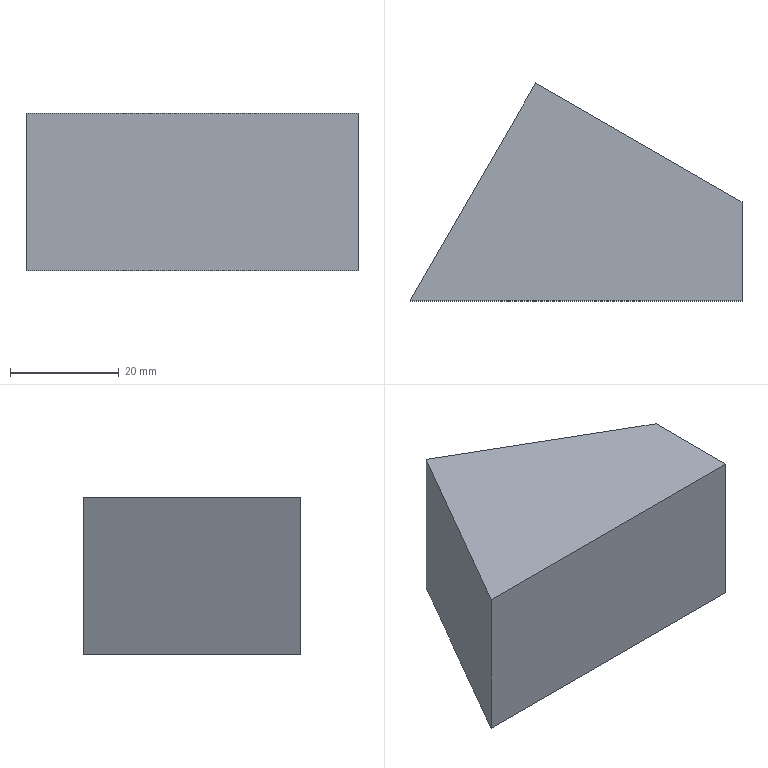Part | Creo | 1 solid | 6 faces | box 61.174 x 40.149 x 29 mm | volume 45647 mm3 | plane 6
STEP:
#1=CARTESIAN_POINT('',(9.022,228.213,-50.5));
#2=VERTEX_POINT('',#1);
#3=CARTESIAN_POINT('',(-28.972,250.149,-50.5));
#4=VERTEX_POINT('',#3);
#5=CARTESIAN_POINT('',(9.022,228.213,-50.5));
#6=DIRECTION('',(-0.866,0.5,0.));
#7=VECTOR('',#6,43.872);
#8=LINE('',#5,#7);
#9=EDGE_CURVE('',#2,#4,#8,.T.);
#10=ORIENTED_EDGE('',*,*,#9,.T.);
#11=CARTESIAN_POINT('',(-28.972,250.149,-79.5));
#12=VERTEX_POINT('',#11);
#13=CARTESIAN_POINT('',(-28.972,250.149,-79.5));
#14=DIRECTION('',(0.,0.,1.));
#15=VECTOR('',#14,29.);
#16=LINE('',#13,#15);
#17=EDGE_CURVE('',#12,#4,#16,.T.);
#18=ORIENTED_EDGE('',*,*,#17,.F.);
#19=CARTESIAN_POINT('',(9.022,228.213,-79.5));
#20=VERTEX_POINT('',#19);
#21=CARTESIAN_POINT('',(-28.972,250.149,-79.5));
#22=DIRECTION('',(0.866,-0.5,0.));
#23=VECTOR('',#22,43.872);
#24=LINE('',#21,#23);
#25=EDGE_CURVE('',#12,#20,#24,.T.);
#26=ORIENTED_EDGE('',*,*,#25,.T.);
#27=CARTESIAN_POINT('',(9.022,228.213,-50.5));
#28=DIRECTION('',(0.,0.,-1.));
#29=VECTOR('',#28,29.);
#30=LINE('',#27,#29);
#31=EDGE_CURVE('',#2,#20,#30,.T.);
#32=ORIENTED_EDGE('',*,*,#31,.F.);
#33=EDGE_LOOP('',(#10,#18,#26,#32));
#34=FACE_OUTER_BOUND('',#33,.F.);
#35=CARTESIAN_POINT('',(-8.145,238.125,-65.));
#36=DIRECTION('',(0.5,0.866,0.));
#37=DIRECTION('',(0.866,-0.5,0.));
#38=AXIS2_PLACEMENT_3D('',#35,#36,#37);
#39=PLANE('',#38);
#40=ADVANCED_FACE('',(#34),#39,.T.);
#41=CARTESIAN_POINT('',(-52.152,210.,-50.5));
#42=VERTEX_POINT('',#41);
#43=CARTESIAN_POINT('',(9.022,210.,-50.5));
#44=VERTEX_POINT('',#43);
#45=CARTESIAN_POINT('',(-52.152,210.,-50.5));
#46=DIRECTION('',(1.,0.,0.));
#47=VECTOR('',#46,61.174);
#48=LINE('',#45,#47);
#49=EDGE_CURVE('',#42,#44,#48,.T.);
#50=ORIENTED_EDGE('',*,*,#49,.F.);
#51=CARTESIAN_POINT('',(-28.972,250.149,-50.5));
#52=DIRECTION('',(-0.5,-0.866,0.));
#53=VECTOR('',#52,46.36);
#54=LINE('',#51,#53);
#55=EDGE_CURVE('',#4,#42,#54,.T.);
#56=ORIENTED_EDGE('',*,*,#55,.F.);
#57=ORIENTED_EDGE('',*,*,#9,.F.);
#58=CARTESIAN_POINT('',(9.022,228.213,-50.5));
#59=DIRECTION('',(0.,-1.,0.));
#60=VECTOR('',#59,18.213);
#61=LINE('',#58,#60);
#62=EDGE_CURVE('',#2,#44,#61,.T.);
#63=ORIENTED_EDGE('',*,*,#62,.T.);
#64=EDGE_LOOP('',(#50,#56,#57,#63));
#65=FACE_OUTER_BOUND('',#64,.F.);
#66=CARTESIAN_POINT('',(-38.495,185.557,-50.5));
#67=DIRECTION('',(0.,0.,1.));
#68=DIRECTION('',(-1.,0.,0.));
#69=AXIS2_PLACEMENT_3D('',#66,#67,#68);
#70=PLANE('',#69);
#71=ADVANCED_FACE('',(#65),#70,.T.);
#72=ORIENTED_EDGE('',*,*,#49,.T.);
#73=CARTESIAN_POINT('',(9.022,210.,-79.5));
#74=VERTEX_POINT('',#73);
#75=CARTESIAN_POINT('',(9.022,210.,-50.5));
#76=DIRECTION('',(0.,0.,-1.));
#77=VECTOR('',#76,29.);
#78=LINE('',#75,#77);
#79=EDGE_CURVE('',#44,#74,#78,.T.);
#80=ORIENTED_EDGE('',*,*,#79,.T.);
#81=CARTESIAN_POINT('',(-52.152,210.,-79.5));
#82=VERTEX_POINT('',#81);
#83=CARTESIAN_POINT('',(9.022,210.,-79.5));
#84=DIRECTION('',(-1.,0.,0.));
#85=VECTOR('',#84,61.174);
#86=LINE('',#83,#85);
#87=EDGE_CURVE('',#74,#82,#86,.T.);
#88=ORIENTED_EDGE('',*,*,#87,.T.);
#89=CARTESIAN_POINT('',(-52.152,210.,-79.5));
#90=DIRECTION('',(0.,0.,1.));
#91=VECTOR('',#90,29.);
#92=LINE('',#89,#91);
#93=EDGE_CURVE('',#82,#42,#92,.T.);
#94=ORIENTED_EDGE('',*,*,#93,.T.);
#95=EDGE_LOOP('',(#72,#80,#88,#94));
#96=FACE_OUTER_BOUND('',#95,.F.);
#97=CARTESIAN_POINT('',(64.87,210.,-2.716));
#98=DIRECTION('',(0.,1.,0.));
#99=DIRECTION('',(-1.,0.,0.));
#100=AXIS2_PLACEMENT_3D('',#97,#98,#99);
#101=PLANE('',#100);
#102=ADVANCED_FACE('',(#96),#101,.F.);
#103=ORIENTED_EDGE('',*,*,#79,.F.);
#104=ORIENTED_EDGE('',*,*,#62,.F.);
#105=ORIENTED_EDGE('',*,*,#31,.T.);
#106=CARTESIAN_POINT('',(9.022,228.213,-79.5));
#107=DIRECTION('',(0.,-1.,0.));
#108=VECTOR('',#107,18.213);
#109=LINE('',#106,#108);
#110=EDGE_CURVE('',#20,#74,#109,.T.);
#111=ORIENTED_EDGE('',*,*,#110,.T.);
#112=EDGE_LOOP('',(#103,#104,#105,#111));
#113=FACE_OUTER_BOUND('',#112,.F.);
#114=CARTESIAN_POINT('',(9.022,231.1,-65.));
#115=DIRECTION('',(1.,0.,0.));
#116=DIRECTION('',(0.,0.,1.));
#117=AXIS2_PLACEMENT_3D('',#114,#115,#116);
#118=PLANE('',#117);
#119=ADVANCED_FACE('',(#113),#118,.T.);
#120=ORIENTED_EDGE('',*,*,#87,.F.);
#121=ORIENTED_EDGE('',*,*,#110,.F.);
#122=ORIENTED_EDGE('',*,*,#25,.F.);
#123=CARTESIAN_POINT('',(-52.152,210.,-79.5));
#124=DIRECTION('',(0.5,0.866,0.));
#125=VECTOR('',#124,46.36);
#126=LINE('',#123,#125);
#127=EDGE_CURVE('',#82,#12,#126,.T.);
#128=ORIENTED_EDGE('',*,*,#127,.F.);
#129=EDGE_LOOP('',(#120,#121,#122,#128));
#130=FACE_OUTER_BOUND('',#129,.F.);
#131=CARTESIAN_POINT('',(-38.495,185.557,-79.5));
#132=DIRECTION('',(0.,0.,-1.));
#133=DIRECTION('',(1.,0.,0.));
#134=AXIS2_PLACEMENT_3D('',#131,#132,#133);
#135=PLANE('',#134);
#136=ADVANCED_FACE('',(#130),#135,.T.);
#137=ORIENTED_EDGE('',*,*,#93,.F.);
#138=ORIENTED_EDGE('',*,*,#127,.T.);
#139=ORIENTED_EDGE('',*,*,#17,.T.);
#140=ORIENTED_EDGE('',*,*,#55,.T.);
#141=EDGE_LOOP('',(#137,#138,#139,#140));
#142=FACE_OUTER_BOUND('',#141,.F.);
#143=CARTESIAN_POINT('',(-59.322,197.581,-65.));
#144=DIRECTION('',(-0.866,0.5,0.));
#145=DIRECTION('',(0.5,0.866,0.));
#146=AXIS2_PLACEMENT_3D('',#143,#144,#145);
#147=PLANE('',#146);
#148=ADVANCED_FACE('',(#142),#147,.T.);
#149=CLOSED_SHELL('',(#40,#71,#102,#119,#136,#148));
#150=MANIFOLD_SOLID_BREP('',#149);
#151=(LENGTH_UNIT()NAMED_UNIT(*)SI_UNIT(.MILLI.,.METRE.));
#152=UNCERTAINTY_MEASURE_WITH_UNIT(LENGTH_MEASURE(0.007871),#151,'','');
#153=(NAMED_UNIT(*)PLANE_ANGLE_UNIT()SI_UNIT($,.RADIAN.));
#154=PLANE_ANGLE_MEASURE_WITH_UNIT(PLANE_ANGLE_MEASURE(0.01745),#153);
#155=(CONVERSION_BASED_UNIT('DEGREE',#154)NAMED_UNIT(*)PLANE_ANGLE_UNIT());
#156=(NAMED_UNIT(*)SI_UNIT($,.STERADIAN.)SOLID_ANGLE_UNIT());
#157=(GEOMETRIC_REPRESENTATION_CONTEXT(3)GLOBAL_UNCERTAINTY_ASSIGNED_CONTEXT((#152))GLOBAL_UNIT_ASSIGNED_CONTEXT((#151,#155,#156))REPRESENTATION_CONTEXT('',''));
#158=ADVANCED_BREP_SHAPE_REPRESENTATION('',(#150),#157);